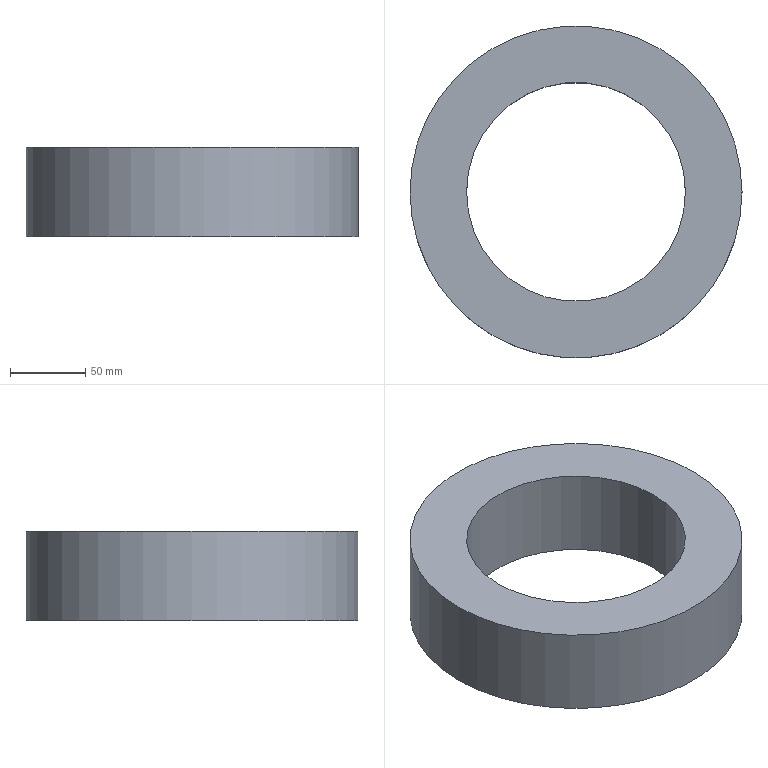Part | NX | features 连杆套筒内 2 | 1 solid | 4 faces | box 220 x 220 x 59.435 mm | volume 1277869 mm3 | plane 2 | cylinder 2 | commonest cylinder face diameters 145 x1 220 x1
STEP:
#1=CARTESIAN_POINT('',(110.,0.,59.435));
#2=VERTEX_POINT('',#1);
#3=CARTESIAN_POINT('',(0.,0.,59.435));
#4=DIRECTION('',(0.,0.,1.));
#5=DIRECTION('',(1.,0.,0.));
#6=AXIS2_PLACEMENT_3D('',#3,#4,#5);
#7=CIRCLE('',#6,110.);
#8=EDGE_CURVE('',#2,#2,#7,.T.);
#9=ORIENTED_EDGE('',*,*,#8,.T.);
#10=EDGE_LOOP('',(#9));
#11=FACE_BOUND('',#10,.T.);
#12=CARTESIAN_POINT('',(72.5,0.,59.435));
#13=VERTEX_POINT('',#12);
#14=CARTESIAN_POINT('',(0.,0.,59.435));
#15=DIRECTION('',(0.,0.,1.));
#16=DIRECTION('',(1.,0.,0.));
#17=AXIS2_PLACEMENT_3D('',#14,#15,#16);
#18=CIRCLE('',#17,72.5);
#19=EDGE_CURVE('',#13,#13,#18,.T.);
#20=ORIENTED_EDGE('',*,*,#19,.F.);
#21=EDGE_LOOP('',(#20));
#22=FACE_BOUND('',#21,.T.);
#23=CARTESIAN_POINT('',(0.,0.,59.435));
#24=DIRECTION('',(0.,0.,1.));
#25=DIRECTION('',(1.,0.,0.));
#26=AXIS2_PLACEMENT_3D('',#23,#24,#25);
#27=PLANE('',#26);
#28=ADVANCED_FACE('',(#11,#22),#27,.T.);
#29=CARTESIAN_POINT('',(110.,0.,0.));
#30=VERTEX_POINT('',#29);
#31=CARTESIAN_POINT('',(0.,0.,0.));
#32=DIRECTION('',(0.,0.,1.));
#33=DIRECTION('',(1.,0.,0.));
#34=AXIS2_PLACEMENT_3D('',#31,#32,#33);
#35=CIRCLE('',#34,110.);
#36=EDGE_CURVE('',#30,#30,#35,.T.);
#37=ORIENTED_EDGE('',*,*,#36,.F.);
#38=EDGE_LOOP('',(#37));
#39=FACE_BOUND('',#38,.T.);
#40=CARTESIAN_POINT('',(72.5,0.,0.));
#41=VERTEX_POINT('',#40);
#42=CARTESIAN_POINT('',(0.,0.,0.));
#43=DIRECTION('',(0.,0.,1.));
#44=DIRECTION('',(1.,0.,0.));
#45=AXIS2_PLACEMENT_3D('',#42,#43,#44);
#46=CIRCLE('',#45,72.5);
#47=EDGE_CURVE('',#41,#41,#46,.T.);
#48=ORIENTED_EDGE('',*,*,#47,.T.);
#49=EDGE_LOOP('',(#48));
#50=FACE_BOUND('',#49,.T.);
#51=CARTESIAN_POINT('',(0.,0.,0.));
#52=DIRECTION('',(0.,0.,1.));
#53=DIRECTION('',(1.,0.,0.));
#54=AXIS2_PLACEMENT_3D('',#51,#52,#53);
#55=PLANE('',#54);
#56=ADVANCED_FACE('',(#39,#50),#55,.F.);
#57=ORIENTED_EDGE('',*,*,#8,.F.);
#58=EDGE_LOOP('',(#57));
#59=FACE_BOUND('',#58,.T.);
#60=ORIENTED_EDGE('',*,*,#36,.T.);
#61=EDGE_LOOP('',(#60));
#62=FACE_BOUND('',#61,.T.);
#63=CARTESIAN_POINT('',(0.,0.,59.435));
#64=DIRECTION('',(0.,0.,-1.));
#65=DIRECTION('',(-1.,0.,0.));
#66=AXIS2_PLACEMENT_3D('',#63,#64,#65);
#67=CYLINDRICAL_SURFACE('',#66,110.);
#68=ADVANCED_FACE('',(#59,#62),#67,.T.);
#69=ORIENTED_EDGE('',*,*,#19,.T.);
#70=EDGE_LOOP('',(#69));
#71=FACE_BOUND('',#70,.T.);
#72=ORIENTED_EDGE('',*,*,#47,.F.);
#73=EDGE_LOOP('',(#72));
#74=FACE_BOUND('',#73,.T.);
#75=CARTESIAN_POINT('',(0.,0.,59.435));
#76=DIRECTION('',(0.,0.,-1.));
#77=DIRECTION('',(-1.,0.,0.));
#78=AXIS2_PLACEMENT_3D('',#75,#76,#77);
#79=CYLINDRICAL_SURFACE('',#78,72.5);
#80=ADVANCED_FACE('',(#71,#74),#79,.F.);
#81=CLOSED_SHELL('',(#28,#56,#68,#80));
#82=MANIFOLD_SOLID_BREP('',#81);
#83=(LENGTH_UNIT()NAMED_UNIT(*)SI_UNIT(.MILLI.,.METRE.));
#84=UNCERTAINTY_MEASURE_WITH_UNIT(LENGTH_MEASURE(0.00001),#83,'','');
#85=(NAMED_UNIT(*)PLANE_ANGLE_UNIT()SI_UNIT($,.RADIAN.));
#86=(NAMED_UNIT(*)SI_UNIT($,.STERADIAN.)SOLID_ANGLE_UNIT());
#87=(GEOMETRIC_REPRESENTATION_CONTEXT(3)GLOBAL_UNCERTAINTY_ASSIGNED_CONTEXT((#84))GLOBAL_UNIT_ASSIGNED_CONTEXT((#83,#85,#86))REPRESENTATION_CONTEXT('',''));
#88=ADVANCED_BREP_SHAPE_REPRESENTATION('',(#82),#87);